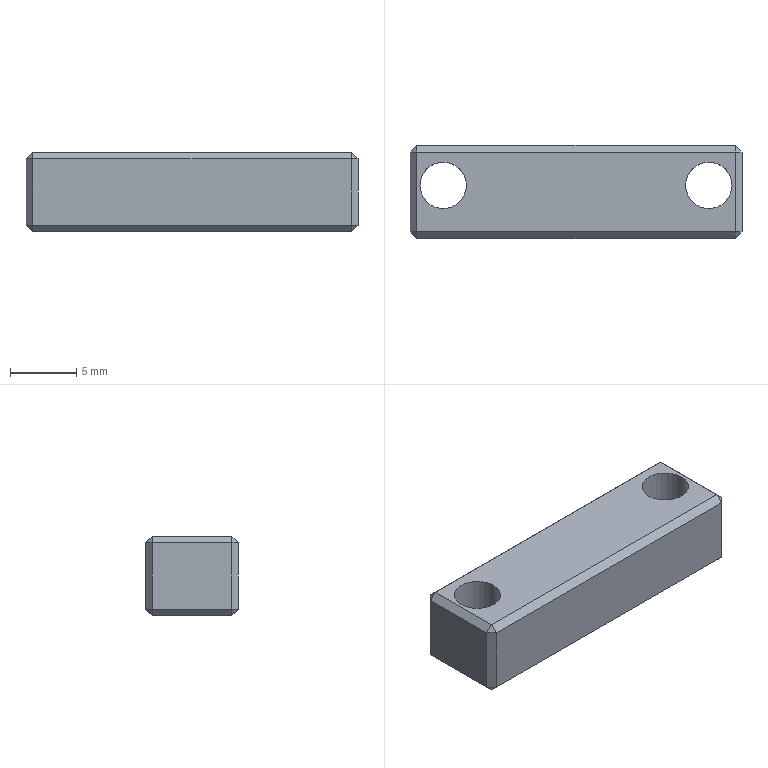Part | SolidWorks | features HoleWzd 2, Chamfer 1, Extrusion 1 | 1 solid | 38 faces | box 25 x 7 x 6 mm | volume 851.742 mm3 | plane 26 | cylinder 8 | cone 4 | commonest cylinder face diameters 3.5 x8
STEP:
#1=CARTESIAN_POINT('',(5.,0.5,0.75));
#2=VERTEX_POINT('',#1);
#3=CARTESIAN_POINT('',(5.,0.5,4.25));
#4=VERTEX_POINT('',#3);
#5=CARTESIAN_POINT('',(5.,0.5,2.5));
#6=DIRECTION('',(0.,1.,0.));
#7=DIRECTION('',(0.,0.,1.));
#8=AXIS2_PLACEMENT_3D('',#5,#6,#7);
#9=CIRCLE('',#8,1.75);
#10=EDGE_CURVE('',#2,#4,#9,.T.);
#11=ORIENTED_EDGE('',*,*,#10,.F.);
#12=CARTESIAN_POINT('',(5.,3.5,0.75));
#13=VERTEX_POINT('',#12);
#14=CARTESIAN_POINT('',(5.,3.5,0.75));
#15=DIRECTION('',(0.,1.,0.));
#16=VECTOR('',#15,1000.);
#17=LINE('',#14,#16);
#18=EDGE_CURVE('',#2,#13,#17,.T.);
#19=ORIENTED_EDGE('',*,*,#18,.T.);
#20=CARTESIAN_POINT('',(5.,3.5,4.25));
#21=VERTEX_POINT('',#20);
#22=CARTESIAN_POINT('',(5.,3.5,2.5));
#23=DIRECTION('',(0.,1.,0.));
#24=DIRECTION('',(0.,0.,1.));
#25=AXIS2_PLACEMENT_3D('',#22,#23,#24);
#26=CIRCLE('',#25,1.75);
#27=EDGE_CURVE('',#13,#21,#26,.T.);
#28=ORIENTED_EDGE('',*,*,#27,.T.);
#29=CARTESIAN_POINT('',(5.,3.5,4.25));
#30=DIRECTION('',(0.,1.,0.));
#31=VECTOR('',#30,1000.);
#32=LINE('',#29,#31);
#33=EDGE_CURVE('',#4,#21,#32,.T.);
#34=ORIENTED_EDGE('',*,*,#33,.F.);
#35=EDGE_LOOP('',(#11,#19,#28,#34));
#36=FACE_OUTER_BOUND('',#35,.T.);
#37=CARTESIAN_POINT('',(5.,3.5,2.5));
#38=DIRECTION('',(0.,1.,0.));
#39=DIRECTION('',(0.,0.,1.));
#40=AXIS2_PLACEMENT_3D('',#37,#38,#39);
#41=CYLINDRICAL_SURFACE('',#40,1.75);
#42=ADVANCED_FACE('',(#36),#41,.F.);
#43=CARTESIAN_POINT('',(5.,-0.5515,2.5));
#44=VERTEX_POINT('',#43);
#45=CARTESIAN_POINT('',(5.,0.5,4.25));
#46=DIRECTION('',(0.,0.515,0.8572));
#47=VECTOR('',#46,1000.);
#48=LINE('',#45,#47);
#49=EDGE_CURVE('',#44,#4,#48,.T.);
#50=ORIENTED_EDGE('',*,*,#49,.F.);
#51=CARTESIAN_POINT('',(5.,0.5,0.75));
#52=DIRECTION('',(0.,0.515,-0.8572));
#53=VECTOR('',#52,1000.);
#54=LINE('',#51,#53);
#55=EDGE_CURVE('',#44,#2,#54,.T.);
#56=ORIENTED_EDGE('',*,*,#55,.T.);
#57=ORIENTED_EDGE('',*,*,#10,.T.);
#58=EDGE_LOOP('',(#50,#56,#57));
#59=FACE_OUTER_BOUND('',#58,.T.);
#60=CARTESIAN_POINT('',(5.,0.5,2.5));
#61=DIRECTION('',(0.,1.,0.));
#62=DIRECTION('',(0.,0.,1.));
#63=AXIS2_PLACEMENT_3D('',#60,#61,#62);
#64=CONICAL_SURFACE('',#63,1.75,1.03);
#65=ADVANCED_FACE('',(#59),#64,.F.);
#66=CARTESIAN_POINT('',(-5.,0.5,0.75));
#67=VERTEX_POINT('',#66);
#68=CARTESIAN_POINT('',(-5.,0.5,4.25));
#69=VERTEX_POINT('',#68);
#70=CARTESIAN_POINT('',(-5.,0.5,2.5));
#71=DIRECTION('',(0.,1.,0.));
#72=DIRECTION('',(0.,0.,1.));
#73=AXIS2_PLACEMENT_3D('',#70,#71,#72);
#74=CIRCLE('',#73,1.75);
#75=EDGE_CURVE('',#67,#69,#74,.T.);
#76=ORIENTED_EDGE('',*,*,#75,.F.);
#77=CARTESIAN_POINT('',(-5.,3.5,0.75));
#78=VERTEX_POINT('',#77);
#79=CARTESIAN_POINT('',(-5.,3.5,0.75));
#80=DIRECTION('',(0.,1.,0.));
#81=VECTOR('',#80,1000.);
#82=LINE('',#79,#81);
#83=EDGE_CURVE('',#67,#78,#82,.T.);
#84=ORIENTED_EDGE('',*,*,#83,.T.);
#85=CARTESIAN_POINT('',(-5.,3.5,4.25));
#86=VERTEX_POINT('',#85);
#87=CARTESIAN_POINT('',(-5.,3.5,2.5));
#88=DIRECTION('',(0.,1.,0.));
#89=DIRECTION('',(0.,0.,1.));
#90=AXIS2_PLACEMENT_3D('',#87,#88,#89);
#91=CIRCLE('',#90,1.75);
#92=EDGE_CURVE('',#78,#86,#91,.T.);
#93=ORIENTED_EDGE('',*,*,#92,.T.);
#94=CARTESIAN_POINT('',(-5.,3.5,4.25));
#95=DIRECTION('',(0.,1.,0.));
#96=VECTOR('',#95,1000.);
#97=LINE('',#94,#96);
#98=EDGE_CURVE('',#69,#86,#97,.T.);
#99=ORIENTED_EDGE('',*,*,#98,.F.);
#100=EDGE_LOOP('',(#76,#84,#93,#99));
#101=FACE_OUTER_BOUND('',#100,.T.);
#102=CARTESIAN_POINT('',(-5.,3.5,2.5));
#103=DIRECTION('',(0.,1.,0.));
#104=DIRECTION('',(0.,0.,1.));
#105=AXIS2_PLACEMENT_3D('',#102,#103,#104);
#106=CYLINDRICAL_SURFACE('',#105,1.75);
#107=ADVANCED_FACE('',(#101),#106,.F.);
#108=CARTESIAN_POINT('',(-5.,-0.5515,2.5));
#109=VERTEX_POINT('',#108);
#110=CARTESIAN_POINT('',(-5.,0.5,4.25));
#111=DIRECTION('',(0.,0.515,0.8572));
#112=VECTOR('',#111,1000.);
#113=LINE('',#110,#112);
#114=EDGE_CURVE('',#109,#69,#113,.T.);
#115=ORIENTED_EDGE('',*,*,#114,.F.);
#116=CARTESIAN_POINT('',(-5.,0.5,0.75));
#117=DIRECTION('',(0.,0.515,-0.8572));
#118=VECTOR('',#117,1000.);
#119=LINE('',#116,#118);
#120=EDGE_CURVE('',#109,#67,#119,.T.);
#121=ORIENTED_EDGE('',*,*,#120,.T.);
#122=ORIENTED_EDGE('',*,*,#75,.T.);
#123=EDGE_LOOP('',(#115,#121,#122));
#124=FACE_OUTER_BOUND('',#123,.T.);
#125=CARTESIAN_POINT('',(-5.,0.5,2.5));
#126=DIRECTION('',(0.,1.,0.));
#127=DIRECTION('',(0.,0.,1.));
#128=AXIS2_PLACEMENT_3D('',#125,#126,#127);
#129=CONICAL_SURFACE('',#128,1.75,1.03);
#130=ADVANCED_FACE('',(#124),#129,.F.);
#131=CARTESIAN_POINT('',(-11.75,0.5,0.));
#132=VERTEX_POINT('',#131);
#133=CARTESIAN_POINT('',(-8.25,0.5,0.));
#134=VERTEX_POINT('',#133);
#135=CARTESIAN_POINT('',(-10.,0.5,0.));
#136=DIRECTION('',(0.,0.,1.));
#137=DIRECTION('',(1.,0.,0.));
#138=AXIS2_PLACEMENT_3D('',#135,#136,#137);
#139=CIRCLE('',#138,1.75);
#140=EDGE_CURVE('',#132,#134,#139,.T.);
#141=ORIENTED_EDGE('',*,*,#140,.F.);
#142=CARTESIAN_POINT('',(-11.75,0.5,6.));
#143=VERTEX_POINT('',#142);
#144=CARTESIAN_POINT('',(-11.75,0.5,6.));
#145=DIRECTION('',(0.,0.,1.));
#146=VECTOR('',#145,1000.);
#147=LINE('',#144,#146);
#148=EDGE_CURVE('',#132,#143,#147,.T.);
#149=ORIENTED_EDGE('',*,*,#148,.T.);
#150=CARTESIAN_POINT('',(-8.25,0.5,6.));
#151=VERTEX_POINT('',#150);
#152=CARTESIAN_POINT('',(-10.,0.5,6.));
#153=DIRECTION('',(0.,0.,1.));
#154=DIRECTION('',(1.,0.,0.));
#155=AXIS2_PLACEMENT_3D('',#152,#153,#154);
#156=CIRCLE('',#155,1.75);
#157=EDGE_CURVE('',#143,#151,#156,.T.);
#158=ORIENTED_EDGE('',*,*,#157,.T.);
#159=CARTESIAN_POINT('',(-8.25,0.5,6.));
#160=DIRECTION('',(0.,0.,1.));
#161=VECTOR('',#160,1000.);
#162=LINE('',#159,#161);
#163=EDGE_CURVE('',#134,#151,#162,.T.);
#164=ORIENTED_EDGE('',*,*,#163,.F.);
#165=EDGE_LOOP('',(#141,#149,#158,#164));
#166=FACE_OUTER_BOUND('',#165,.T.);
#167=CARTESIAN_POINT('',(-10.,0.5,6.));
#168=DIRECTION('',(0.,0.,1.));
#169=DIRECTION('',(1.,0.,0.));
#170=AXIS2_PLACEMENT_3D('',#167,#168,#169);
#171=CYLINDRICAL_SURFACE('',#170,1.75);
#172=ADVANCED_FACE('',(#166),#171,.F.);
#173=CARTESIAN_POINT('',(8.25,0.5,0.));
#174=VERTEX_POINT('',#173);
#175=CARTESIAN_POINT('',(11.75,0.5,0.));
#176=VERTEX_POINT('',#175);
#177=CARTESIAN_POINT('',(10.,0.5,0.));
#178=DIRECTION('',(0.,0.,1.));
#179=DIRECTION('',(1.,0.,0.));
#180=AXIS2_PLACEMENT_3D('',#177,#178,#179);
#181=CIRCLE('',#180,1.75);
#182=EDGE_CURVE('',#174,#176,#181,.T.);
#183=ORIENTED_EDGE('',*,*,#182,.F.);
#184=CARTESIAN_POINT('',(8.25,0.5,6.));
#185=VERTEX_POINT('',#184);
#186=CARTESIAN_POINT('',(8.25,0.5,6.));
#187=DIRECTION('',(0.,0.,1.));
#188=VECTOR('',#187,1000.);
#189=LINE('',#186,#188);
#190=EDGE_CURVE('',#174,#185,#189,.T.);
#191=ORIENTED_EDGE('',*,*,#190,.T.);
#192=CARTESIAN_POINT('',(11.75,0.5,6.));
#193=VERTEX_POINT('',#192);
#194=CARTESIAN_POINT('',(10.,0.5,6.));
#195=DIRECTION('',(0.,0.,1.));
#196=DIRECTION('',(1.,0.,0.));
#197=AXIS2_PLACEMENT_3D('',#194,#195,#196);
#198=CIRCLE('',#197,1.75);
#199=EDGE_CURVE('',#185,#193,#198,.T.);
#200=ORIENTED_EDGE('',*,*,#199,.T.);
#201=CARTESIAN_POINT('',(11.75,0.5,6.));
#202=DIRECTION('',(0.,0.,1.));
#203=VECTOR('',#202,1000.);
#204=LINE('',#201,#203);
#205=EDGE_CURVE('',#176,#193,#204,.T.);
#206=ORIENTED_EDGE('',*,*,#205,.F.);
#207=EDGE_LOOP('',(#183,#191,#200,#206));
#208=FACE_OUTER_BOUND('',#207,.T.);
#209=CARTESIAN_POINT('',(10.,0.5,6.));
#210=DIRECTION('',(0.,0.,1.));
#211=DIRECTION('',(1.,0.,0.));
#212=AXIS2_PLACEMENT_3D('',#209,#210,#211);
#213=CYLINDRICAL_SURFACE('',#212,1.75);
#214=ADVANCED_FACE('',(#208),#213,.F.);
#215=CARTESIAN_POINT('',(12.5,-3.,5.5));
#216=VERTEX_POINT('',#215);
#217=CARTESIAN_POINT('',(12.5,-3.,0.5));
#218=VERTEX_POINT('',#217);
#219=CARTESIAN_POINT('',(12.5,-3.,6.));
#220=DIRECTION('',(0.,0.,-1.));
#221=VECTOR('',#220,1000.);
#222=LINE('',#219,#221);
#223=EDGE_CURVE('',#216,#218,#222,.T.);
#224=ORIENTED_EDGE('',*,*,#223,.T.);
#225=CARTESIAN_POINT('',(12.5,3.,0.5));
#226=VERTEX_POINT('',#225);
#227=CARTESIAN_POINT('',(12.5,3.5,0.5));
#228=DIRECTION('',(0.,1.,0.));
#229=VECTOR('',#228,1000.);
#230=LINE('',#227,#229);
#231=EDGE_CURVE('',#218,#226,#230,.T.);
#232=ORIENTED_EDGE('',*,*,#231,.T.);
#233=CARTESIAN_POINT('',(12.5,3.,5.5));
#234=VERTEX_POINT('',#233);
#235=CARTESIAN_POINT('',(12.5,3.,6.));
#236=DIRECTION('',(0.,0.,1.));
#237=VECTOR('',#236,1000.);
#238=LINE('',#235,#237);
#239=EDGE_CURVE('',#226,#234,#238,.T.);
#240=ORIENTED_EDGE('',*,*,#239,.T.);
#241=CARTESIAN_POINT('',(12.5,-3.5,5.5));
#242=DIRECTION('',(0.,-1.,0.));
#243=VECTOR('',#242,1000.);
#244=LINE('',#241,#243);
#245=EDGE_CURVE('',#234,#216,#244,.T.);
#246=ORIENTED_EDGE('',*,*,#245,.T.);
#247=EDGE_LOOP('',(#224,#232,#240,#246));
#248=FACE_OUTER_BOUND('',#247,.T.);
#249=CARTESIAN_POINT('',(12.5,-3.5,6.));
#250=DIRECTION('',(-1.,0.,0.));
#251=DIRECTION('',(0.,0.,1.));
#252=AXIS2_PLACEMENT_3D('',#249,#250,#251);
#253=PLANE('',#252);
#254=ADVANCED_FACE('',(#248),#253,.F.);
#255=CARTESIAN_POINT('',(12.,3.5,5.5));
#256=VERTEX_POINT('',#255);
#257=CARTESIAN_POINT('',(12.,3.5,0.5));
#258=VERTEX_POINT('',#257);
#259=CARTESIAN_POINT('',(12.,3.5,6.));
#260=DIRECTION('',(0.,0.,-1.));
#261=VECTOR('',#260,1000.);
#262=LINE('',#259,#261);
#263=EDGE_CURVE('',#256,#258,#262,.T.);
#264=ORIENTED_EDGE('',*,*,#263,.T.);
#265=CARTESIAN_POINT('',(-12.,3.5,0.5));
#266=VERTEX_POINT('',#265);
#267=CARTESIAN_POINT('',(-12.5,3.5,0.5));
#268=DIRECTION('',(-1.,0.,0.));
#269=VECTOR('',#268,1000.);
#270=LINE('',#267,#269);
#271=EDGE_CURVE('',#258,#266,#270,.T.);
#272=ORIENTED_EDGE('',*,*,#271,.T.);
#273=CARTESIAN_POINT('',(-12.,3.5,5.5));
#274=VERTEX_POINT('',#273);
#275=CARTESIAN_POINT('',(-12.,3.5,6.));
#276=DIRECTION('',(0.,0.,1.));
#277=VECTOR('',#276,1000.);
#278=LINE('',#275,#277);
#279=EDGE_CURVE('',#266,#274,#278,.T.);
#280=ORIENTED_EDGE('',*,*,#279,.T.);
#281=CARTESIAN_POINT('',(-12.5,3.5,5.5));
#282=DIRECTION('',(1.,0.,0.));
#283=VECTOR('',#282,1000.);
#284=LINE('',#281,#283);
#285=EDGE_CURVE('',#274,#256,#284,.T.);
#286=ORIENTED_EDGE('',*,*,#285,.T.);
#287=EDGE_LOOP('',(#264,#272,#280,#286));
#288=FACE_OUTER_BOUND('',#287,.T.);
#289=CARTESIAN_POINT('',(5.,3.5,2.5));
#290=DIRECTION('',(0.,1.,0.));
#291=DIRECTION('',(0.,0.,1.));
#292=AXIS2_PLACEMENT_3D('',#289,#290,#291);
#293=CIRCLE('',#292,1.75);
#294=EDGE_CURVE('',#21,#13,#293,.T.);
#295=ORIENTED_EDGE('',*,*,#294,.F.);
#296=ORIENTED_EDGE('',*,*,#27,.F.);
#297=EDGE_LOOP('',(#295,#296));
#298=FACE_BOUND('',#297,.T.);
#299=CARTESIAN_POINT('',(-5.,3.5,2.5));
#300=DIRECTION('',(0.,1.,0.));
#301=DIRECTION('',(0.,0.,1.));
#302=AXIS2_PLACEMENT_3D('',#299,#300,#301);
#303=CIRCLE('',#302,1.75);
#304=EDGE_CURVE('',#86,#78,#303,.T.);
#305=ORIENTED_EDGE('',*,*,#304,.F.);
#306=ORIENTED_EDGE('',*,*,#92,.F.);
#307=EDGE_LOOP('',(#305,#306));
#308=FACE_BOUND('',#307,.T.);
#309=CARTESIAN_POINT('',(-12.5,3.5,6.));
#310=DIRECTION('',(0.,-1.,0.));
#311=DIRECTION('',(0.,0.,-1.));
#312=AXIS2_PLACEMENT_3D('',#309,#310,#311);
#313=PLANE('',#312);
#314=ADVANCED_FACE('',(#288,#298,#308),#313,.F.);
#315=CARTESIAN_POINT('',(-12.5,3.,5.5));
#316=VERTEX_POINT('',#315);
#317=CARTESIAN_POINT('',(-12.5,3.,0.5));
#318=VERTEX_POINT('',#317);
#319=CARTESIAN_POINT('',(-12.5,3.,6.));
#320=DIRECTION('',(0.,0.,-1.));
#321=VECTOR('',#320,1000.);
#322=LINE('',#319,#321);
#323=EDGE_CURVE('',#316,#318,#322,.T.);
#324=ORIENTED_EDGE('',*,*,#323,.T.);
#325=CARTESIAN_POINT('',(-12.5,-3.,0.5));
#326=VERTEX_POINT('',#325);
#327=CARTESIAN_POINT('',(-12.5,-3.5,0.5));
#328=DIRECTION('',(0.,-1.,0.));
#329=VECTOR('',#328,1000.);
#330=LINE('',#327,#329);
#331=EDGE_CURVE('',#318,#326,#330,.T.);
#332=ORIENTED_EDGE('',*,*,#331,.T.);
#333=CARTESIAN_POINT('',(-12.5,-3.,5.5));
#334=VERTEX_POINT('',#333);
#335=CARTESIAN_POINT('',(-12.5,-3.,6.));
#336=DIRECTION('',(0.,0.,1.));
#337=VECTOR('',#336,1000.);
#338=LINE('',#335,#337);
#339=EDGE_CURVE('',#326,#334,#338,.T.);
#340=ORIENTED_EDGE('',*,*,#339,.T.);
#341=CARTESIAN_POINT('',(-12.5,-3.5,5.5));
#342=DIRECTION('',(0.,1.,0.));
#343=VECTOR('',#342,1000.);
#344=LINE('',#341,#343);
#345=EDGE_CURVE('',#334,#316,#344,.T.);
#346=ORIENTED_EDGE('',*,*,#345,.T.);
#347=EDGE_LOOP('',(#324,#332,#340,#346));
#348=FACE_OUTER_BOUND('',#347,.T.);
#349=CARTESIAN_POINT('',(-12.5,-3.5,6.));
#350=DIRECTION('',(1.,0.,0.));
#351=DIRECTION('',(0.,0.,-1.));
#352=AXIS2_PLACEMENT_3D('',#349,#350,#351);
#353=PLANE('',#352);
#354=ADVANCED_FACE('',(#348),#353,.F.);
#355=CARTESIAN_POINT('',(-12.,-3.5,5.5));
#356=VERTEX_POINT('',#355);
#357=CARTESIAN_POINT('',(-12.,-3.5,0.5));
#358=VERTEX_POINT('',#357);
#359=CARTESIAN_POINT('',(-12.,-3.5,6.));
#360=DIRECTION('',(0.,0.,-1.));
#361=VECTOR('',#360,1000.);
#362=LINE('',#359,#361);
#363=EDGE_CURVE('',#356,#358,#362,.T.);
#364=ORIENTED_EDGE('',*,*,#363,.T.);
#365=CARTESIAN_POINT('',(12.,-3.5,0.5));
#366=VERTEX_POINT('',#365);
#367=CARTESIAN_POINT('',(12.5,-3.5,0.5));
#368=DIRECTION('',(1.,0.,0.));
#369=VECTOR('',#368,1000.);
#370=LINE('',#367,#369);
#371=EDGE_CURVE('',#358,#366,#370,.T.);
#372=ORIENTED_EDGE('',*,*,#371,.T.);
#373=CARTESIAN_POINT('',(12.,-3.5,5.5));
#374=VERTEX_POINT('',#373);
#375=CARTESIAN_POINT('',(12.,-3.5,6.));
#376=DIRECTION('',(0.,0.,1.));
#377=VECTOR('',#376,1000.);
#378=LINE('',#375,#377);
#379=EDGE_CURVE('',#366,#374,#378,.T.);
#380=ORIENTED_EDGE('',*,*,#379,.T.);
#381=CARTESIAN_POINT('',(-12.5,-3.5,5.5));
#382=DIRECTION('',(-1.,0.,0.));
#383=VECTOR('',#382,1000.);
#384=LINE('',#381,#383);
#385=EDGE_CURVE('',#374,#356,#384,.T.);
#386=ORIENTED_EDGE('',*,*,#385,.T.);
#387=EDGE_LOOP('',(#364,#372,#380,#386));
#388=FACE_OUTER_BOUND('',#387,.T.);
#389=CARTESIAN_POINT('',(-12.5,-3.5,6.));
#390=DIRECTION('',(0.,1.,0.));
#391=DIRECTION('',(0.,0.,1.));
#392=AXIS2_PLACEMENT_3D('',#389,#390,#391);
#393=PLANE('',#392);
#394=ADVANCED_FACE('',(#388),#393,.F.);
#395=CARTESIAN_POINT('',(12.,3.,6.));
#396=VERTEX_POINT('',#395);
#397=CARTESIAN_POINT('',(-12.,3.,6.));
#398=VERTEX_POINT('',#397);
#399=CARTESIAN_POINT('',(0.,3.,6.));
#400=DIRECTION('',(-1.,0.,0.));
#401=VECTOR('',#400,1000.);
#402=LINE('',#399,#401);
#403=EDGE_CURVE('',#396,#398,#402,.T.);
#404=ORIENTED_EDGE('',*,*,#403,.T.);
#405=CARTESIAN_POINT('',(-12.,-3.,6.));
#406=VERTEX_POINT('',#405);
#407=CARTESIAN_POINT('',(-12.,0.,6.));
#408=DIRECTION('',(0.,-1.,0.));
#409=VECTOR('',#408,1000.);
#410=LINE('',#407,#409);
#411=EDGE_CURVE('',#398,#406,#410,.T.);
#412=ORIENTED_EDGE('',*,*,#411,.T.);
#413=CARTESIAN_POINT('',(12.,-3.,6.));
#414=VERTEX_POINT('',#413);
#415=CARTESIAN_POINT('',(0.,-3.,6.));
#416=DIRECTION('',(1.,0.,0.));
#417=VECTOR('',#416,1000.);
#418=LINE('',#415,#417);
#419=EDGE_CURVE('',#406,#414,#418,.T.);
#420=ORIENTED_EDGE('',*,*,#419,.T.);
#421=CARTESIAN_POINT('',(12.,0.,6.));
#422=DIRECTION('',(0.,1.,0.));
#423=VECTOR('',#422,1000.);
#424=LINE('',#421,#423);
#425=EDGE_CURVE('',#414,#396,#424,.T.);
#426=ORIENTED_EDGE('',*,*,#425,.T.);
#427=EDGE_LOOP('',(#404,#412,#420,#426));
#428=FACE_OUTER_BOUND('',#427,.T.);
#429=CARTESIAN_POINT('',(-10.,0.5,6.));
#430=DIRECTION('',(0.,0.,1.));
#431=DIRECTION('',(1.,0.,0.));
#432=AXIS2_PLACEMENT_3D('',#429,#430,#431);
#433=CIRCLE('',#432,1.75);
#434=EDGE_CURVE('',#151,#143,#433,.T.);
#435=ORIENTED_EDGE('',*,*,#434,.F.);
#436=ORIENTED_EDGE('',*,*,#157,.F.);
#437=EDGE_LOOP('',(#435,#436));
#438=FACE_BOUND('',#437,.T.);
#439=CARTESIAN_POINT('',(10.,0.5,6.));
#440=DIRECTION('',(0.,0.,1.));
#441=DIRECTION('',(1.,0.,0.));
#442=AXIS2_PLACEMENT_3D('',#439,#440,#441);
#443=CIRCLE('',#442,1.75);
#444=EDGE_CURVE('',#193,#185,#443,.T.);
#445=ORIENTED_EDGE('',*,*,#444,.F.);
#446=ORIENTED_EDGE('',*,*,#199,.F.);
#447=EDGE_LOOP('',(#445,#446));
#448=FACE_BOUND('',#447,.T.);
#449=CARTESIAN_POINT('',(0.,0.,6.));
#450=DIRECTION('',(0.,0.,-1.));
#451=DIRECTION('',(-1.,0.,0.));
#452=AXIS2_PLACEMENT_3D('',#449,#450,#451);
#453=PLANE('',#452);
#454=ADVANCED_FACE('',(#428,#438,#448),#453,.F.);
#455=CARTESIAN_POINT('',(12.,3.,0.));
#456=VERTEX_POINT('',#455);
#457=CARTESIAN_POINT('',(12.,-3.,0.));
#458=VERTEX_POINT('',#457);
#459=CARTESIAN_POINT('',(12.,-3.5,0.));
#460=DIRECTION('',(0.,-1.,0.));
#461=VECTOR('',#460,1000.);
#462=LINE('',#459,#461);
#463=EDGE_CURVE('',#456,#458,#462,.T.);
#464=ORIENTED_EDGE('',*,*,#463,.T.);
#465=CARTESIAN_POINT('',(-12.,-3.,0.));
#466=VERTEX_POINT('',#465);
#467=CARTESIAN_POINT('',(-12.5,-3.,0.));
#468=DIRECTION('',(-1.,0.,0.));
#469=VECTOR('',#468,1000.);
#470=LINE('',#467,#469);
#471=EDGE_CURVE('',#458,#466,#470,.T.);
#472=ORIENTED_EDGE('',*,*,#471,.T.);
#473=CARTESIAN_POINT('',(-12.,3.,0.));
#474=VERTEX_POINT('',#473);
#475=CARTESIAN_POINT('',(-12.,3.5,0.));
#476=DIRECTION('',(0.,1.,0.));
#477=VECTOR('',#476,1000.);
#478=LINE('',#475,#477);
#479=EDGE_CURVE('',#466,#474,#478,.T.);
#480=ORIENTED_EDGE('',*,*,#479,.T.);
#481=CARTESIAN_POINT('',(12.5,3.,0.));
#482=DIRECTION('',(1.,0.,0.));
#483=VECTOR('',#482,1000.);
#484=LINE('',#481,#483);
#485=EDGE_CURVE('',#474,#456,#484,.T.);
#486=ORIENTED_EDGE('',*,*,#485,.T.);
#487=EDGE_LOOP('',(#464,#472,#480,#486));
#488=FACE_OUTER_BOUND('',#487,.T.);
#489=CARTESIAN_POINT('',(-10.,0.5,0.));
#490=DIRECTION('',(0.,0.,1.));
#491=DIRECTION('',(1.,0.,0.));
#492=AXIS2_PLACEMENT_3D('',#489,#490,#491);
#493=CIRCLE('',#492,1.75);
#494=EDGE_CURVE('',#134,#132,#493,.T.);
#495=ORIENTED_EDGE('',*,*,#494,.T.);
#496=ORIENTED_EDGE('',*,*,#140,.T.);
#497=EDGE_LOOP('',(#495,#496));
#498=FACE_BOUND('',#497,.T.);
#499=CARTESIAN_POINT('',(10.,0.5,0.));
#500=DIRECTION('',(0.,0.,1.));
#501=DIRECTION('',(1.,0.,0.));
#502=AXIS2_PLACEMENT_3D('',#499,#500,#501);
#503=CIRCLE('',#502,1.75);
#504=EDGE_CURVE('',#176,#174,#503,.T.);
#505=ORIENTED_EDGE('',*,*,#504,.T.);
#506=ORIENTED_EDGE('',*,*,#182,.T.);
#507=EDGE_LOOP('',(#505,#506));
#508=FACE_BOUND('',#507,.T.);
#509=CARTESIAN_POINT('',(0.,0.,0.));
#510=DIRECTION('',(0.,0.,-1.));
#511=DIRECTION('',(-1.,0.,0.));
#512=AXIS2_PLACEMENT_3D('',#509,#510,#511);
#513=PLANE('',#512);
#514=ADVANCED_FACE('',(#488,#498,#508),#513,.T.);
#515=ORIENTED_EDGE('',*,*,#190,.F.);
#516=ORIENTED_EDGE('',*,*,#504,.F.);
#517=ORIENTED_EDGE('',*,*,#205,.T.);
#518=ORIENTED_EDGE('',*,*,#444,.T.);
#519=EDGE_LOOP('',(#515,#516,#517,#518));
#520=FACE_OUTER_BOUND('',#519,.T.);
#521=CARTESIAN_POINT('',(10.,0.5,6.));
#522=DIRECTION('',(0.,0.,1.));
#523=DIRECTION('',(1.,0.,0.));
#524=AXIS2_PLACEMENT_3D('',#521,#522,#523);
#525=CYLINDRICAL_SURFACE('',#524,1.75);
#526=ADVANCED_FACE('',(#520),#525,.F.);
#527=ORIENTED_EDGE('',*,*,#148,.F.);
#528=ORIENTED_EDGE('',*,*,#494,.F.);
#529=ORIENTED_EDGE('',*,*,#163,.T.);
#530=ORIENTED_EDGE('',*,*,#434,.T.);
#531=EDGE_LOOP('',(#527,#528,#529,#530));
#532=FACE_OUTER_BOUND('',#531,.T.);
#533=CARTESIAN_POINT('',(-10.,0.5,6.));
#534=DIRECTION('',(0.,0.,1.));
#535=DIRECTION('',(1.,0.,0.));
#536=AXIS2_PLACEMENT_3D('',#533,#534,#535);
#537=CYLINDRICAL_SURFACE('',#536,1.75);
#538=ADVANCED_FACE('',(#532),#537,.F.);
#539=ORIENTED_EDGE('',*,*,#120,.F.);
#540=ORIENTED_EDGE('',*,*,#114,.T.);
#541=CARTESIAN_POINT('',(-5.,0.5,2.5));
#542=DIRECTION('',(0.,1.,0.));
#543=DIRECTION('',(0.,0.,1.));
#544=AXIS2_PLACEMENT_3D('',#541,#542,#543);
#545=CIRCLE('',#544,1.75);
#546=EDGE_CURVE('',#69,#67,#545,.T.);
#547=ORIENTED_EDGE('',*,*,#546,.T.);
#548=EDGE_LOOP('',(#539,#540,#547));
#549=FACE_OUTER_BOUND('',#548,.T.);
#550=CARTESIAN_POINT('',(-5.,0.5,2.5));
#551=DIRECTION('',(0.,1.,0.));
#552=DIRECTION('',(0.,0.,1.));
#553=AXIS2_PLACEMENT_3D('',#550,#551,#552);
#554=CONICAL_SURFACE('',#553,1.75,1.03);
#555=ADVANCED_FACE('',(#549),#554,.F.);
#556=ORIENTED_EDGE('',*,*,#83,.F.);
#557=ORIENTED_EDGE('',*,*,#546,.F.);
#558=ORIENTED_EDGE('',*,*,#98,.T.);
#559=ORIENTED_EDGE('',*,*,#304,.T.);
#560=EDGE_LOOP('',(#556,#557,#558,#559));
#561=FACE_OUTER_BOUND('',#560,.T.);
#562=CARTESIAN_POINT('',(-5.,3.5,2.5));
#563=DIRECTION('',(0.,1.,0.));
#564=DIRECTION('',(0.,0.,1.));
#565=AXIS2_PLACEMENT_3D('',#562,#563,#564);
#566=CYLINDRICAL_SURFACE('',#565,1.75);
#567=ADVANCED_FACE('',(#561),#566,.F.);
#568=ORIENTED_EDGE('',*,*,#55,.F.);
#569=ORIENTED_EDGE('',*,*,#49,.T.);
#570=CARTESIAN_POINT('',(5.,0.5,2.5));
#571=DIRECTION('',(0.,1.,0.));
#572=DIRECTION('',(0.,0.,1.));
#573=AXIS2_PLACEMENT_3D('',#570,#571,#572);
#574=CIRCLE('',#573,1.75);
#575=EDGE_CURVE('',#4,#2,#574,.T.);
#576=ORIENTED_EDGE('',*,*,#575,.T.);
#577=EDGE_LOOP('',(#568,#569,#576));
#578=FACE_OUTER_BOUND('',#577,.T.);
#579=CARTESIAN_POINT('',(5.,0.5,2.5));
#580=DIRECTION('',(0.,1.,0.));
#581=DIRECTION('',(0.,0.,1.));
#582=AXIS2_PLACEMENT_3D('',#579,#580,#581);
#583=CONICAL_SURFACE('',#582,1.75,1.03);
#584=ADVANCED_FACE('',(#578),#583,.F.);
#585=ORIENTED_EDGE('',*,*,#18,.F.);
#586=ORIENTED_EDGE('',*,*,#575,.F.);
#587=ORIENTED_EDGE('',*,*,#33,.T.);
#588=ORIENTED_EDGE('',*,*,#294,.T.);
#589=EDGE_LOOP('',(#585,#586,#587,#588));
#590=FACE_OUTER_BOUND('',#589,.T.);
#591=CARTESIAN_POINT('',(5.,3.5,2.5));
#592=DIRECTION('',(0.,1.,0.));
#593=DIRECTION('',(0.,0.,1.));
#594=AXIS2_PLACEMENT_3D('',#591,#592,#593);
#595=CYLINDRICAL_SURFACE('',#594,1.75);
#596=ADVANCED_FACE('',(#590),#595,.F.);
#597=CARTESIAN_POINT('',(-12.,3.5,5.5));
#598=DIRECTION('',(0.,0.7071,-0.7071));
#599=VECTOR('',#598,1000.);
#600=LINE('',#597,#599);
#601=EDGE_CURVE('',#398,#274,#600,.T.);
#602=ORIENTED_EDGE('',*,*,#601,.F.);
#603=ORIENTED_EDGE('',*,*,#403,.F.);
#604=CARTESIAN_POINT('',(12.,3.25,5.75));
#605=DIRECTION('',(0.,-0.7071,0.7071));
#606=VECTOR('',#605,1000.);
#607=LINE('',#604,#606);
#608=EDGE_CURVE('',#256,#396,#607,.T.);
#609=ORIENTED_EDGE('',*,*,#608,.F.);
#610=ORIENTED_EDGE('',*,*,#285,.F.);
#611=EDGE_LOOP('',(#602,#603,#609,#610));
#612=FACE_OUTER_BOUND('',#611,.T.);
#613=CARTESIAN_POINT('',(0.,3.,6.));
#614=DIRECTION('',(0.,-0.7071,-0.7071));
#615=DIRECTION('',(-1.,0.,0.));
#616=AXIS2_PLACEMENT_3D('',#613,#614,#615);
#617=PLANE('',#616);
#618=ADVANCED_FACE('',(#612),#617,.F.);
#619=CARTESIAN_POINT('',(-12.25,3.,5.75));
#620=DIRECTION('',(-0.7071,0.,-0.7071));
#621=VECTOR('',#620,1000.);
#622=LINE('',#619,#621);
#623=EDGE_CURVE('',#398,#316,#622,.T.);
#624=ORIENTED_EDGE('',*,*,#623,.F.);
#625=ORIENTED_EDGE('',*,*,#601,.T.);
#626=CARTESIAN_POINT('',(-12.,3.5,5.5));
#627=DIRECTION('',(0.7071,0.7071,0.));
#628=VECTOR('',#627,1000.);
#629=LINE('',#626,#628);
#630=EDGE_CURVE('',#316,#274,#629,.T.);
#631=ORIENTED_EDGE('',*,*,#630,.F.);
#632=EDGE_LOOP('',(#624,#625,#631));
#633=FACE_OUTER_BOUND('',#632,.T.);
#634=CARTESIAN_POINT('',(-12.,3.5,5.5));
#635=DIRECTION('',(-0.5774,0.5774,0.5774));
#636=DIRECTION('',(-0.7071,-0.7071,0.));
#637=AXIS2_PLACEMENT_3D('',#634,#635,#636);
#638=PLANE('',#637);
#639=ADVANCED_FACE('',(#633),#638,.T.);
#640=CARTESIAN_POINT('',(12.5,3.,5.5));
#641=DIRECTION('',(0.7071,-0.7071,0.));
#642=VECTOR('',#641,1000.);
#643=LINE('',#640,#642);
#644=EDGE_CURVE('',#256,#234,#643,.T.);
#645=ORIENTED_EDGE('',*,*,#644,.F.);
#646=ORIENTED_EDGE('',*,*,#608,.T.);
#647=CARTESIAN_POINT('',(12.5,3.,5.5));
#648=DIRECTION('',(-0.7071,0.,0.7071));
#649=VECTOR('',#648,1000.);
#650=LINE('',#647,#649);
#651=EDGE_CURVE('',#234,#396,#650,.T.);
#652=ORIENTED_EDGE('',*,*,#651,.F.);
#653=EDGE_LOOP('',(#645,#646,#652));
#654=FACE_OUTER_BOUND('',#653,.T.);
#655=CARTESIAN_POINT('',(12.5,3.,5.5));
#656=DIRECTION('',(0.5774,0.5774,0.5774));
#657=DIRECTION('',(-0.7071,0.7071,0.));
#658=AXIS2_PLACEMENT_3D('',#655,#656,#657);
#659=PLANE('',#658);
#660=ADVANCED_FACE('',(#654),#659,.T.);
#661=ORIENTED_EDGE('',*,*,#630,.T.);
#662=ORIENTED_EDGE('',*,*,#279,.F.);
#663=CARTESIAN_POINT('',(-12.25,3.25,0.5));
#664=DIRECTION('',(0.7071,0.7071,0.));
#665=VECTOR('',#664,1000.);
#666=LINE('',#663,#665);
#667=EDGE_CURVE('',#318,#266,#666,.T.);
#668=ORIENTED_EDGE('',*,*,#667,.F.);
#669=ORIENTED_EDGE('',*,*,#323,.F.);
#670=EDGE_LOOP('',(#661,#662,#668,#669));
#671=FACE_OUTER_BOUND('',#670,.T.);
#672=CARTESIAN_POINT('',(-12.5,3.,6.));
#673=DIRECTION('',(0.7071,-0.7071,0.));
#674=DIRECTION('',(0.,0.,-1.));
#675=AXIS2_PLACEMENT_3D('',#672,#673,#674);
#676=PLANE('',#675);
#677=ADVANCED_FACE('',(#671),#676,.F.);
#678=ORIENTED_EDGE('',*,*,#623,.T.);
#679=ORIENTED_EDGE('',*,*,#345,.F.);
#680=CARTESIAN_POINT('',(-12.5,-3.,5.5));
#681=DIRECTION('',(-0.7071,0.,-0.7071));
#682=VECTOR('',#681,1000.);
#683=LINE('',#680,#682);
#684=EDGE_CURVE('',#406,#334,#683,.T.);
#685=ORIENTED_EDGE('',*,*,#684,.F.);
#686=ORIENTED_EDGE('',*,*,#411,.F.);
#687=EDGE_LOOP('',(#678,#679,#685,#686));
#688=FACE_OUTER_BOUND('',#687,.T.);
#689=CARTESIAN_POINT('',(-12.,0.,6.));
#690=DIRECTION('',(0.7071,0.,-0.7071));
#691=DIRECTION('',(0.,-1.,0.));
#692=AXIS2_PLACEMENT_3D('',#689,#690,#691);
#693=PLANE('',#692);
#694=ADVANCED_FACE('',(#688),#693,.F.);
#695=CARTESIAN_POINT('',(12.,-3.5,5.5));
#696=DIRECTION('',(0.,-0.7071,-0.7071));
#697=VECTOR('',#696,1000.);
#698=LINE('',#695,#697);
#699=EDGE_CURVE('',#414,#374,#698,.T.);
#700=ORIENTED_EDGE('',*,*,#699,.F.);
#701=ORIENTED_EDGE('',*,*,#419,.F.);
#702=CARTESIAN_POINT('',(-12.,-3.25,5.75));
#703=DIRECTION('',(0.,0.7071,0.7071));
#704=VECTOR('',#703,1000.);
#705=LINE('',#702,#704);
#706=EDGE_CURVE('',#356,#406,#705,.T.);
#707=ORIENTED_EDGE('',*,*,#706,.F.);
#708=ORIENTED_EDGE('',*,*,#385,.F.);
#709=EDGE_LOOP('',(#700,#701,#707,#708));
#710=FACE_OUTER_BOUND('',#709,.T.);
#711=CARTESIAN_POINT('',(0.,-3.,6.));
#712=DIRECTION('',(0.,0.7071,-0.7071));
#713=DIRECTION('',(1.,0.,0.));
#714=AXIS2_PLACEMENT_3D('',#711,#712,#713);
#715=PLANE('',#714);
#716=ADVANCED_FACE('',(#710),#715,.F.);
#717=ORIENTED_EDGE('',*,*,#651,.T.);
#718=ORIENTED_EDGE('',*,*,#425,.F.);
#719=CARTESIAN_POINT('',(12.25,-3.,5.75));
#720=DIRECTION('',(-0.7071,0.,0.7071));
#721=VECTOR('',#720,1000.);
#722=LINE('',#719,#721);
#723=EDGE_CURVE('',#216,#414,#722,.T.);
#724=ORIENTED_EDGE('',*,*,#723,.F.);
#725=ORIENTED_EDGE('',*,*,#245,.F.);
#726=EDGE_LOOP('',(#717,#718,#724,#725));
#727=FACE_OUTER_BOUND('',#726,.T.);
#728=CARTESIAN_POINT('',(12.,0.,6.));
#729=DIRECTION('',(-0.7071,0.,-0.7071));
#730=DIRECTION('',(0.,1.,0.));
#731=AXIS2_PLACEMENT_3D('',#728,#729,#730);
#732=PLANE('',#731);
#733=ADVANCED_FACE('',(#727),#732,.F.);
#734=ORIENTED_EDGE('',*,*,#644,.T.);
#735=ORIENTED_EDGE('',*,*,#239,.F.);
#736=CARTESIAN_POINT('',(12.5,3.,0.5));
#737=DIRECTION('',(0.7071,-0.7071,0.));
#738=VECTOR('',#737,1000.);
#739=LINE('',#736,#738);
#740=EDGE_CURVE('',#258,#226,#739,.T.);
#741=ORIENTED_EDGE('',*,*,#740,.F.);
#742=ORIENTED_EDGE('',*,*,#263,.F.);
#743=EDGE_LOOP('',(#734,#735,#741,#742));
#744=FACE_OUTER_BOUND('',#743,.T.);
#745=CARTESIAN_POINT('',(12.,3.5,6.));
#746=DIRECTION('',(-0.7071,-0.7071,0.));
#747=DIRECTION('',(0.,0.,-1.));
#748=AXIS2_PLACEMENT_3D('',#745,#746,#747);
#749=PLANE('',#748);
#750=ADVANCED_FACE('',(#744),#749,.F.);
#751=CARTESIAN_POINT('',(-12.,3.,0.));
#752=DIRECTION('',(0.,-0.7071,-0.7071));
#753=VECTOR('',#752,1000.);
#754=LINE('',#751,#753);
#755=EDGE_CURVE('',#266,#474,#754,.T.);
#756=ORIENTED_EDGE('',*,*,#755,.F.);
#757=ORIENTED_EDGE('',*,*,#271,.F.);
#758=CARTESIAN_POINT('',(12.,3.25,0.25));
#759=DIRECTION('',(0.,0.7071,0.7071));
#760=VECTOR('',#759,1000.);
#761=LINE('',#758,#760);
#762=EDGE_CURVE('',#456,#258,#761,.T.);
#763=ORIENTED_EDGE('',*,*,#762,.F.);
#764=ORIENTED_EDGE('',*,*,#485,.F.);
#765=EDGE_LOOP('',(#756,#757,#763,#764));
#766=FACE_OUTER_BOUND('',#765,.T.);
#767=CARTESIAN_POINT('',(-12.5,3.5,0.5));
#768=DIRECTION('',(0.,0.7071,-0.7071));
#769=DIRECTION('',(1.,0.,0.));
#770=AXIS2_PLACEMENT_3D('',#767,#768,#769);
#771=PLANE('',#770);
#772=ADVANCED_FACE('',(#766),#771,.T.);
#773=ORIENTED_EDGE('',*,*,#667,.T.);
#774=ORIENTED_EDGE('',*,*,#755,.T.);
#775=CARTESIAN_POINT('',(-12.,3.,0.));
#776=DIRECTION('',(0.7071,0.,-0.7071));
#777=VECTOR('',#776,1000.);
#778=LINE('',#775,#777);
#779=EDGE_CURVE('',#318,#474,#778,.T.);
#780=ORIENTED_EDGE('',*,*,#779,.F.);
#781=EDGE_LOOP('',(#773,#774,#780));
#782=FACE_OUTER_BOUND('',#781,.T.);
#783=CARTESIAN_POINT('',(-12.,3.,0.));
#784=DIRECTION('',(-0.5774,0.5774,-0.5774));
#785=DIRECTION('',(0.,0.7071,0.7071));
#786=AXIS2_PLACEMENT_3D('',#783,#784,#785);
#787=PLANE('',#786);
#788=ADVANCED_FACE('',(#782),#787,.T.);
#789=ORIENTED_EDGE('',*,*,#706,.T.);
#790=ORIENTED_EDGE('',*,*,#684,.T.);
#791=CARTESIAN_POINT('',(-12.5,-3.,5.5));
#792=DIRECTION('',(-0.7071,0.7071,0.));
#793=VECTOR('',#792,1000.);
#794=LINE('',#791,#793);
#795=EDGE_CURVE('',#356,#334,#794,.T.);
#796=ORIENTED_EDGE('',*,*,#795,.F.);
#797=EDGE_LOOP('',(#789,#790,#796));
#798=FACE_OUTER_BOUND('',#797,.T.);
#799=CARTESIAN_POINT('',(-12.5,-3.,5.5));
#800=DIRECTION('',(-0.5774,-0.5774,0.5774));
#801=DIRECTION('',(0.7071,-0.7071,0.));
#802=AXIS2_PLACEMENT_3D('',#799,#800,#801);
#803=PLANE('',#802);
#804=ADVANCED_FACE('',(#798),#803,.T.);
#805=ORIENTED_EDGE('',*,*,#723,.T.);
#806=ORIENTED_EDGE('',*,*,#699,.T.);
#807=CARTESIAN_POINT('',(12.,-3.5,5.5));
#808=DIRECTION('',(-0.7071,-0.7071,0.));
#809=VECTOR('',#808,1000.);
#810=LINE('',#807,#809);
#811=EDGE_CURVE('',#216,#374,#810,.T.);
#812=ORIENTED_EDGE('',*,*,#811,.F.);
#813=EDGE_LOOP('',(#805,#806,#812));
#814=FACE_OUTER_BOUND('',#813,.T.);
#815=CARTESIAN_POINT('',(12.,-3.5,5.5));
#816=DIRECTION('',(0.5774,-0.5774,0.5774));
#817=DIRECTION('',(0.7071,0.7071,0.));
#818=AXIS2_PLACEMENT_3D('',#815,#816,#817);
#819=PLANE('',#818);
#820=ADVANCED_FACE('',(#814),#819,.T.);
#821=ORIENTED_EDGE('',*,*,#762,.T.);
#822=ORIENTED_EDGE('',*,*,#740,.T.);
#823=CARTESIAN_POINT('',(12.5,3.,0.5));
#824=DIRECTION('',(0.7071,0.,0.7071));
#825=VECTOR('',#824,1000.);
#826=LINE('',#823,#825);
#827=EDGE_CURVE('',#456,#226,#826,.T.);
#828=ORIENTED_EDGE('',*,*,#827,.F.);
#829=EDGE_LOOP('',(#821,#822,#828));
#830=FACE_OUTER_BOUND('',#829,.T.);
#831=CARTESIAN_POINT('',(12.5,3.,0.5));
#832=DIRECTION('',(0.5774,0.5774,-0.5774));
#833=DIRECTION('',(-0.7071,0.,-0.7071));
#834=AXIS2_PLACEMENT_3D('',#831,#832,#833);
#835=PLANE('',#834);
#836=ADVANCED_FACE('',(#830),#835,.T.);
#837=ORIENTED_EDGE('',*,*,#779,.T.);
#838=ORIENTED_EDGE('',*,*,#479,.F.);
#839=CARTESIAN_POINT('',(-12.,-3.,0.));
#840=DIRECTION('',(0.7071,0.,-0.7071));
#841=VECTOR('',#840,1000.);
#842=LINE('',#839,#841);
#843=EDGE_CURVE('',#326,#466,#842,.T.);
#844=ORIENTED_EDGE('',*,*,#843,.F.);
#845=ORIENTED_EDGE('',*,*,#331,.F.);
#846=EDGE_LOOP('',(#837,#838,#844,#845));
#847=FACE_OUTER_BOUND('',#846,.T.);
#848=CARTESIAN_POINT('',(-12.5,-3.5,0.5));
#849=DIRECTION('',(-0.7071,0.,-0.7071));
#850=DIRECTION('',(0.,1.,0.));
#851=AXIS2_PLACEMENT_3D('',#848,#849,#850);
#852=PLANE('',#851);
#853=ADVANCED_FACE('',(#847),#852,.T.);
#854=ORIENTED_EDGE('',*,*,#795,.T.);
#855=ORIENTED_EDGE('',*,*,#339,.F.);
#856=CARTESIAN_POINT('',(-12.25,-3.25,0.5));
#857=DIRECTION('',(-0.7071,0.7071,0.));
#858=VECTOR('',#857,1000.);
#859=LINE('',#856,#858);
#860=EDGE_CURVE('',#358,#326,#859,.T.);
#861=ORIENTED_EDGE('',*,*,#860,.F.);
#862=ORIENTED_EDGE('',*,*,#363,.F.);
#863=EDGE_LOOP('',(#854,#855,#861,#862));
#864=FACE_OUTER_BOUND('',#863,.T.);
#865=CARTESIAN_POINT('',(-12.,-3.5,6.));
#866=DIRECTION('',(0.7071,0.7071,0.));
#867=DIRECTION('',(0.,0.,-1.));
#868=AXIS2_PLACEMENT_3D('',#865,#866,#867);
#869=PLANE('',#868);
#870=ADVANCED_FACE('',(#864),#869,.F.);
#871=ORIENTED_EDGE('',*,*,#811,.T.);
#872=ORIENTED_EDGE('',*,*,#379,.F.);
#873=CARTESIAN_POINT('',(12.,-3.5,0.5));
#874=DIRECTION('',(-0.7071,-0.7071,0.));
#875=VECTOR('',#874,1000.);
#876=LINE('',#873,#875);
#877=EDGE_CURVE('',#218,#366,#876,.T.);
#878=ORIENTED_EDGE('',*,*,#877,.F.);
#879=ORIENTED_EDGE('',*,*,#223,.F.);
#880=EDGE_LOOP('',(#871,#872,#878,#879));
#881=FACE_OUTER_BOUND('',#880,.T.);
#882=CARTESIAN_POINT('',(12.5,-3.,6.));
#883=DIRECTION('',(-0.7071,0.7071,0.));
#884=DIRECTION('',(0.,0.,-1.));
#885=AXIS2_PLACEMENT_3D('',#882,#883,#884);
#886=PLANE('',#885);
#887=ADVANCED_FACE('',(#881),#886,.F.);
#888=ORIENTED_EDGE('',*,*,#827,.T.);
#889=ORIENTED_EDGE('',*,*,#231,.F.);
#890=CARTESIAN_POINT('',(12.25,-3.,0.25));
#891=DIRECTION('',(0.7071,0.,0.7071));
#892=VECTOR('',#891,1000.);
#893=LINE('',#890,#892);
#894=EDGE_CURVE('',#458,#218,#893,.T.);
#895=ORIENTED_EDGE('',*,*,#894,.F.);
#896=ORIENTED_EDGE('',*,*,#463,.F.);
#897=EDGE_LOOP('',(#888,#889,#895,#896));
#898=FACE_OUTER_BOUND('',#897,.T.);
#899=CARTESIAN_POINT('',(12.5,-3.5,0.5));
#900=DIRECTION('',(0.7071,0.,-0.7071));
#901=DIRECTION('',(0.,-1.,0.));
#902=AXIS2_PLACEMENT_3D('',#899,#900,#901);
#903=PLANE('',#902);
#904=ADVANCED_FACE('',(#898),#903,.T.);
#905=ORIENTED_EDGE('',*,*,#860,.T.);
#906=ORIENTED_EDGE('',*,*,#843,.T.);
#907=CARTESIAN_POINT('',(-12.,-3.,0.));
#908=DIRECTION('',(0.,0.7071,-0.7071));
#909=VECTOR('',#908,1000.);
#910=LINE('',#907,#909);
#911=EDGE_CURVE('',#358,#466,#910,.T.);
#912=ORIENTED_EDGE('',*,*,#911,.F.);
#913=EDGE_LOOP('',(#905,#906,#912));
#914=FACE_OUTER_BOUND('',#913,.T.);
#915=CARTESIAN_POINT('',(-12.,-3.,0.));
#916=DIRECTION('',(-0.5774,-0.5774,-0.5774));
#917=DIRECTION('',(0.,0.7071,-0.7071));
#918=AXIS2_PLACEMENT_3D('',#915,#916,#917);
#919=PLANE('',#918);
#920=ADVANCED_FACE('',(#914),#919,.T.);
#921=ORIENTED_EDGE('',*,*,#894,.T.);
#922=ORIENTED_EDGE('',*,*,#877,.T.);
#923=CARTESIAN_POINT('',(12.,-3.5,0.5));
#924=DIRECTION('',(0.,-0.7071,0.7071));
#925=VECTOR('',#924,1000.);
#926=LINE('',#923,#925);
#927=EDGE_CURVE('',#458,#366,#926,.T.);
#928=ORIENTED_EDGE('',*,*,#927,.F.);
#929=EDGE_LOOP('',(#921,#922,#928));
#930=FACE_OUTER_BOUND('',#929,.T.);
#931=CARTESIAN_POINT('',(12.,-3.5,0.5));
#932=DIRECTION('',(0.5774,-0.5774,-0.5774));
#933=DIRECTION('',(0.,0.7071,-0.7071));
#934=AXIS2_PLACEMENT_3D('',#931,#932,#933);
#935=PLANE('',#934);
#936=ADVANCED_FACE('',(#930),#935,.T.);
#937=ORIENTED_EDGE('',*,*,#911,.T.);
#938=ORIENTED_EDGE('',*,*,#471,.F.);
#939=ORIENTED_EDGE('',*,*,#927,.T.);
#940=ORIENTED_EDGE('',*,*,#371,.F.);
#941=EDGE_LOOP('',(#937,#938,#939,#940));
#942=FACE_OUTER_BOUND('',#941,.T.);
#943=CARTESIAN_POINT('',(-12.5,-3.5,0.5));
#944=DIRECTION('',(0.,-0.7071,-0.7071));
#945=DIRECTION('',(-1.,0.,0.));
#946=AXIS2_PLACEMENT_3D('',#943,#944,#945);
#947=PLANE('',#946);
#948=ADVANCED_FACE('',(#942),#947,.T.);
#949=CLOSED_SHELL('',(#42,#65,#107,#130,#172,#214,#254,#314,#354,#394,#454,#514,#526,#538,#555,#567,#584,#596,#618,#639,#660,#677,#694,#716,#733,#750,#772,#788,#804,#820,#836,#853,#870,#887,#904,#920,#936,#948));
#950=MANIFOLD_SOLID_BREP('',#949);
#951=CARTESIAN_POINT('',(0.,0.,0.));
#952=DIRECTION('',(0.,0.,1.));
#953=DIRECTION('',(1.,0.,0.));
#954=AXIS2_PLACEMENT_3D('',#951,#952,#953);
#955=(LENGTH_UNIT()NAMED_UNIT(*)SI_UNIT(.MILLI.,.METRE.));
#956=UNCERTAINTY_MEASURE_WITH_UNIT(LENGTH_MEASURE(0.00001),#955,'','');
#957=(NAMED_UNIT(*)PLANE_ANGLE_UNIT()SI_UNIT($,.RADIAN.));
#958=(NAMED_UNIT(*)SI_UNIT($,.STERADIAN.)SOLID_ANGLE_UNIT());
#959=(GEOMETRIC_REPRESENTATION_CONTEXT(3)GLOBAL_UNCERTAINTY_ASSIGNED_CONTEXT((#956))GLOBAL_UNIT_ASSIGNED_CONTEXT((#955,#957,#958))REPRESENTATION_CONTEXT('',''));
#960=ADVANCED_BREP_SHAPE_REPRESENTATION('',(#950,#954),#959);